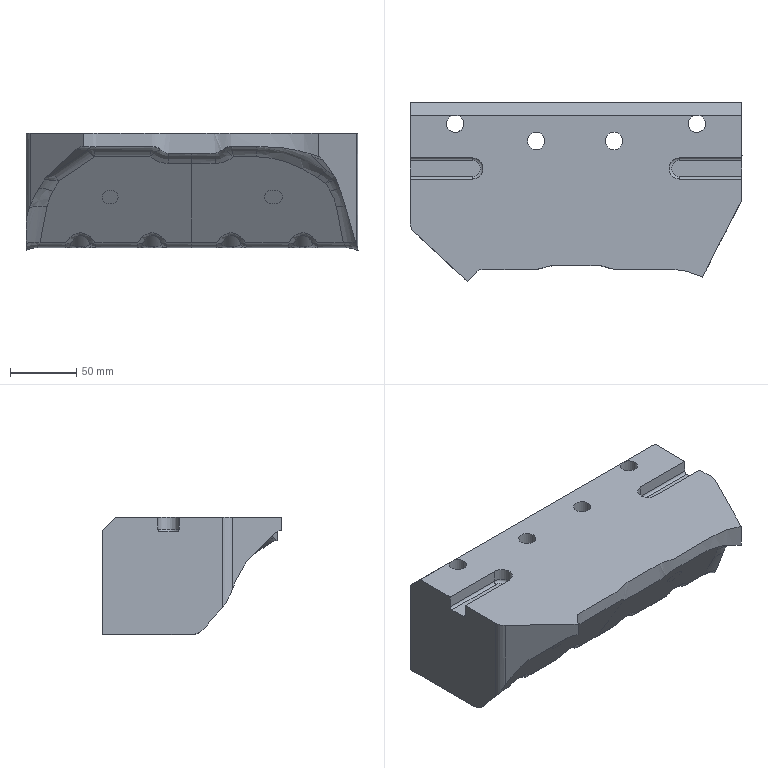Part | NX | features solid 2 | 1 solid | 114 faces | box 250.001 x 134.808 x 88.473 mm | volume 1871431 mm3 | cylinder 43 | spline 41 | plane 25 | cone 2 | torus 2 | sphere 1 | commonest cylinder face diameters 15 x6 32 x6 35 x6 20 x5 4 x4 13 x4